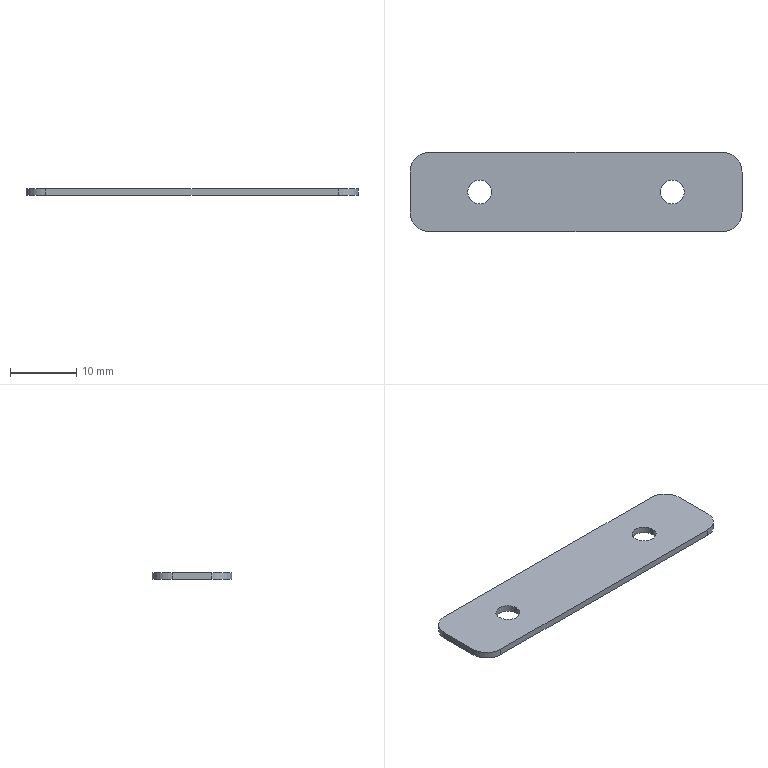Part | NX | features BREP 1 | 1 solid | 14 faces | box 50 x 12 x 1 mm | volume 571.917 mm3 | cylinder 8 | plane 6 | commonest cylinder face diameters 3.6 x4 6 x4
STEP:
#1=CARTESIAN_POINT('',(-22.,6.,1.));
#2=VERTEX_POINT('',#1);
#3=CARTESIAN_POINT('',(-25.,3.,1.));
#4=VERTEX_POINT('',#3);
#5=CARTESIAN_POINT('',(-22.,3.,1.));
#6=DIRECTION('',(0.,0.,1.));
#7=DIRECTION('',(-1.,0.,0.));
#8=AXIS2_PLACEMENT_3D('',#5,#6,#7);
#9=CIRCLE('',#8,3.);
#10=EDGE_CURVE('',#2,#4,#9,.T.);
#11=ORIENTED_EDGE('',*,*,#10,.F.);
#12=CARTESIAN_POINT('',(-22.,6.,0.));
#13=VERTEX_POINT('',#12);
#14=CARTESIAN_POINT('',(-22.,6.,1.));
#15=DIRECTION('',(0.,0.,1.));
#16=VECTOR('',#15,1000.);
#17=LINE('',#14,#16);
#18=EDGE_CURVE('',#13,#2,#17,.T.);
#19=ORIENTED_EDGE('',*,*,#18,.F.);
#20=CARTESIAN_POINT('',(-25.,3.,0.));
#21=VERTEX_POINT('',#20);
#22=CARTESIAN_POINT('',(-22.,3.,0.));
#23=DIRECTION('',(0.,0.,-1.));
#24=DIRECTION('',(-1.,0.,0.));
#25=AXIS2_PLACEMENT_3D('',#22,#23,#24);
#26=CIRCLE('',#25,3.);
#27=EDGE_CURVE('',#21,#13,#26,.T.);
#28=ORIENTED_EDGE('',*,*,#27,.F.);
#29=CARTESIAN_POINT('',(-25.,3.,1.));
#30=DIRECTION('',(0.,0.,-1.));
#31=VECTOR('',#30,1000.);
#32=LINE('',#29,#31);
#33=EDGE_CURVE('',#4,#21,#32,.T.);
#34=ORIENTED_EDGE('',*,*,#33,.F.);
#35=EDGE_LOOP('',(#11,#19,#28,#34));
#36=FACE_BOUND('',#35,.T.);
#37=CARTESIAN_POINT('',(-22.,3.,1.));
#38=DIRECTION('',(0.,0.,-1.));
#39=DIRECTION('',(-1.,0.,0.));
#40=AXIS2_PLACEMENT_3D('',#37,#38,#39);
#41=CYLINDRICAL_SURFACE('',#40,3.);
#42=ADVANCED_FACE('',(#36),#41,.T.);
#43=CARTESIAN_POINT('',(-25.,-3.,1.));
#44=VERTEX_POINT('',#43);
#45=CARTESIAN_POINT('',(-22.,-6.,1.));
#46=VERTEX_POINT('',#45);
#47=CARTESIAN_POINT('',(-22.,-3.,1.));
#48=DIRECTION('',(0.,0.,1.));
#49=DIRECTION('',(-1.,0.,0.));
#50=AXIS2_PLACEMENT_3D('',#47,#48,#49);
#51=CIRCLE('',#50,3.);
#52=EDGE_CURVE('',#44,#46,#51,.T.);
#53=ORIENTED_EDGE('',*,*,#52,.F.);
#54=CARTESIAN_POINT('',(-25.,-3.,0.));
#55=VERTEX_POINT('',#54);
#56=CARTESIAN_POINT('',(-25.,-3.,1.));
#57=DIRECTION('',(0.,0.,1.));
#58=VECTOR('',#57,1000.);
#59=LINE('',#56,#58);
#60=EDGE_CURVE('',#55,#44,#59,.T.);
#61=ORIENTED_EDGE('',*,*,#60,.F.);
#62=CARTESIAN_POINT('',(-22.,-6.,0.));
#63=VERTEX_POINT('',#62);
#64=CARTESIAN_POINT('',(-22.,-3.,0.));
#65=DIRECTION('',(0.,0.,-1.));
#66=DIRECTION('',(-1.,0.,0.));
#67=AXIS2_PLACEMENT_3D('',#64,#65,#66);
#68=CIRCLE('',#67,3.);
#69=EDGE_CURVE('',#63,#55,#68,.T.);
#70=ORIENTED_EDGE('',*,*,#69,.F.);
#71=CARTESIAN_POINT('',(-22.,-6.,1.));
#72=DIRECTION('',(0.,0.,-1.));
#73=VECTOR('',#72,1000.);
#74=LINE('',#71,#73);
#75=EDGE_CURVE('',#46,#63,#74,.T.);
#76=ORIENTED_EDGE('',*,*,#75,.F.);
#77=EDGE_LOOP('',(#53,#61,#70,#76));
#78=FACE_BOUND('',#77,.T.);
#79=CARTESIAN_POINT('',(-22.,-3.,1.));
#80=DIRECTION('',(0.,0.,-1.));
#81=DIRECTION('',(-1.,0.,0.));
#82=AXIS2_PLACEMENT_3D('',#79,#80,#81);
#83=CYLINDRICAL_SURFACE('',#82,3.);
#84=ADVANCED_FACE('',(#78),#83,.T.);
#85=CARTESIAN_POINT('',(25.,3.,1.));
#86=VERTEX_POINT('',#85);
#87=CARTESIAN_POINT('',(22.,6.,1.));
#88=VERTEX_POINT('',#87);
#89=CARTESIAN_POINT('',(22.,3.,1.));
#90=DIRECTION('',(0.,0.,1.));
#91=DIRECTION('',(-1.,0.,0.));
#92=AXIS2_PLACEMENT_3D('',#89,#90,#91);
#93=CIRCLE('',#92,3.);
#94=EDGE_CURVE('',#86,#88,#93,.T.);
#95=ORIENTED_EDGE('',*,*,#94,.F.);
#96=CARTESIAN_POINT('',(25.,3.,0.));
#97=VERTEX_POINT('',#96);
#98=CARTESIAN_POINT('',(25.,3.,1.));
#99=DIRECTION('',(0.,0.,1.));
#100=VECTOR('',#99,1000.);
#101=LINE('',#98,#100);
#102=EDGE_CURVE('',#97,#86,#101,.T.);
#103=ORIENTED_EDGE('',*,*,#102,.F.);
#104=CARTESIAN_POINT('',(22.,6.,0.));
#105=VERTEX_POINT('',#104);
#106=CARTESIAN_POINT('',(22.,3.,0.));
#107=DIRECTION('',(0.,0.,-1.));
#108=DIRECTION('',(-1.,0.,0.));
#109=AXIS2_PLACEMENT_3D('',#106,#107,#108);
#110=CIRCLE('',#109,3.);
#111=EDGE_CURVE('',#105,#97,#110,.T.);
#112=ORIENTED_EDGE('',*,*,#111,.F.);
#113=CARTESIAN_POINT('',(22.,6.,1.));
#114=DIRECTION('',(0.,0.,-1.));
#115=VECTOR('',#114,1000.);
#116=LINE('',#113,#115);
#117=EDGE_CURVE('',#88,#105,#116,.T.);
#118=ORIENTED_EDGE('',*,*,#117,.F.);
#119=EDGE_LOOP('',(#95,#103,#112,#118));
#120=FACE_BOUND('',#119,.T.);
#121=CARTESIAN_POINT('',(22.,3.,1.));
#122=DIRECTION('',(0.,0.,-1.));
#123=DIRECTION('',(-1.,0.,0.));
#124=AXIS2_PLACEMENT_3D('',#121,#122,#123);
#125=CYLINDRICAL_SURFACE('',#124,3.);
#126=ADVANCED_FACE('',(#120),#125,.T.);
#127=CARTESIAN_POINT('',(22.,-6.,1.));
#128=VERTEX_POINT('',#127);
#129=CARTESIAN_POINT('',(25.,-3.,1.));
#130=VERTEX_POINT('',#129);
#131=CARTESIAN_POINT('',(22.,-3.,1.));
#132=DIRECTION('',(0.,0.,1.));
#133=DIRECTION('',(-1.,0.,0.));
#134=AXIS2_PLACEMENT_3D('',#131,#132,#133);
#135=CIRCLE('',#134,3.);
#136=EDGE_CURVE('',#128,#130,#135,.T.);
#137=ORIENTED_EDGE('',*,*,#136,.F.);
#138=CARTESIAN_POINT('',(22.,-6.,0.));
#139=VERTEX_POINT('',#138);
#140=CARTESIAN_POINT('',(22.,-6.,1.));
#141=DIRECTION('',(0.,0.,1.));
#142=VECTOR('',#141,1000.);
#143=LINE('',#140,#142);
#144=EDGE_CURVE('',#139,#128,#143,.T.);
#145=ORIENTED_EDGE('',*,*,#144,.F.);
#146=CARTESIAN_POINT('',(25.,-3.,0.));
#147=VERTEX_POINT('',#146);
#148=CARTESIAN_POINT('',(22.,-3.,0.));
#149=DIRECTION('',(0.,0.,-1.));
#150=DIRECTION('',(-1.,0.,0.));
#151=AXIS2_PLACEMENT_3D('',#148,#149,#150);
#152=CIRCLE('',#151,3.);
#153=EDGE_CURVE('',#147,#139,#152,.T.);
#154=ORIENTED_EDGE('',*,*,#153,.F.);
#155=CARTESIAN_POINT('',(25.,-3.,1.));
#156=DIRECTION('',(0.,0.,-1.));
#157=VECTOR('',#156,1000.);
#158=LINE('',#155,#157);
#159=EDGE_CURVE('',#130,#147,#158,.T.);
#160=ORIENTED_EDGE('',*,*,#159,.F.);
#161=EDGE_LOOP('',(#137,#145,#154,#160));
#162=FACE_BOUND('',#161,.T.);
#163=CARTESIAN_POINT('',(22.,-3.,1.));
#164=DIRECTION('',(0.,0.,-1.));
#165=DIRECTION('',(-1.,0.,0.));
#166=AXIS2_PLACEMENT_3D('',#163,#164,#165);
#167=CYLINDRICAL_SURFACE('',#166,3.);
#168=ADVANCED_FACE('',(#162),#167,.T.);
#169=CARTESIAN_POINT('',(12.7,0.,1.));
#170=VERTEX_POINT('',#169);
#171=CARTESIAN_POINT('',(12.7,0.,0.));
#172=VERTEX_POINT('',#171);
#173=CARTESIAN_POINT('',(12.7,0.,0.));
#174=DIRECTION('',(0.,0.,1.));
#175=VECTOR('',#174,1000.);
#176=LINE('',#173,#175);
#177=EDGE_CURVE('',#170,#172,#176,.F.);
#178=ORIENTED_EDGE('',*,*,#177,.T.);
#179=CARTESIAN_POINT('',(16.3,0.,0.));
#180=VERTEX_POINT('',#179);
#181=CARTESIAN_POINT('',(14.5,0.,0.));
#182=DIRECTION('',(0.,0.,1.));
#183=DIRECTION('',(1.,0.,0.));
#184=AXIS2_PLACEMENT_3D('',#181,#182,#183);
#185=CIRCLE('',#184,1.8);
#186=EDGE_CURVE('',#180,#172,#185,.T.);
#187=ORIENTED_EDGE('',*,*,#186,.F.);
#188=CARTESIAN_POINT('',(16.3,0.,1.));
#189=VERTEX_POINT('',#188);
#190=CARTESIAN_POINT('',(16.3,0.,0.));
#191=DIRECTION('',(0.,0.,1.));
#192=VECTOR('',#191,1000.);
#193=LINE('',#190,#192);
#194=EDGE_CURVE('',#189,#180,#193,.F.);
#195=ORIENTED_EDGE('',*,*,#194,.F.);
#196=CARTESIAN_POINT('',(14.5,0.,1.));
#197=DIRECTION('',(0.,0.,1.));
#198=DIRECTION('',(1.,0.,0.));
#199=AXIS2_PLACEMENT_3D('',#196,#197,#198);
#200=CIRCLE('',#199,1.8);
#201=EDGE_CURVE('',#189,#170,#200,.T.);
#202=ORIENTED_EDGE('',*,*,#201,.T.);
#203=EDGE_LOOP('',(#178,#187,#195,#202));
#204=FACE_BOUND('',#203,.T.);
#205=CARTESIAN_POINT('',(14.5,0.,0.));
#206=DIRECTION('',(0.,0.,1.));
#207=DIRECTION('',(1.,0.,0.));
#208=AXIS2_PLACEMENT_3D('',#205,#206,#207);
#209=CYLINDRICAL_SURFACE('',#208,1.8);
#210=ADVANCED_FACE('',(#204),#209,.F.);
#211=CARTESIAN_POINT('',(-16.3,0.,1.));
#212=VERTEX_POINT('',#211);
#213=CARTESIAN_POINT('',(-16.3,0.,0.));
#214=VERTEX_POINT('',#213);
#215=CARTESIAN_POINT('',(-16.3,0.,0.));
#216=DIRECTION('',(0.,0.,1.));
#217=VECTOR('',#216,1000.);
#218=LINE('',#215,#217);
#219=EDGE_CURVE('',#212,#214,#218,.F.);
#220=ORIENTED_EDGE('',*,*,#219,.T.);
#221=CARTESIAN_POINT('',(-12.7,0.,0.));
#222=VERTEX_POINT('',#221);
#223=CARTESIAN_POINT('',(-14.5,0.,0.));
#224=DIRECTION('',(0.,0.,1.));
#225=DIRECTION('',(1.,0.,0.));
#226=AXIS2_PLACEMENT_3D('',#223,#224,#225);
#227=CIRCLE('',#226,1.8);
#228=EDGE_CURVE('',#222,#214,#227,.T.);
#229=ORIENTED_EDGE('',*,*,#228,.F.);
#230=CARTESIAN_POINT('',(-12.7,0.,1.));
#231=VERTEX_POINT('',#230);
#232=CARTESIAN_POINT('',(-12.7,0.,0.));
#233=DIRECTION('',(0.,0.,1.));
#234=VECTOR('',#233,1000.);
#235=LINE('',#232,#234);
#236=EDGE_CURVE('',#231,#222,#235,.F.);
#237=ORIENTED_EDGE('',*,*,#236,.F.);
#238=CARTESIAN_POINT('',(-14.5,0.,1.));
#239=DIRECTION('',(0.,0.,1.));
#240=DIRECTION('',(1.,0.,0.));
#241=AXIS2_PLACEMENT_3D('',#238,#239,#240);
#242=CIRCLE('',#241,1.8);
#243=EDGE_CURVE('',#231,#212,#242,.T.);
#244=ORIENTED_EDGE('',*,*,#243,.T.);
#245=EDGE_LOOP('',(#220,#229,#237,#244));
#246=FACE_BOUND('',#245,.T.);
#247=CARTESIAN_POINT('',(-14.5,0.,0.));
#248=DIRECTION('',(0.,0.,1.));
#249=DIRECTION('',(1.,0.,0.));
#250=AXIS2_PLACEMENT_3D('',#247,#248,#249);
#251=CYLINDRICAL_SURFACE('',#250,1.8);
#252=ADVANCED_FACE('',(#246),#251,.F.);
#253=CARTESIAN_POINT('',(25.,-6.,0.));
#254=DIRECTION('',(0.,1.,0.));
#255=VECTOR('',#254,1000.);
#256=LINE('',#253,#255);
#257=EDGE_CURVE('',#147,#97,#256,.T.);
#258=ORIENTED_EDGE('',*,*,#257,.F.);
#259=ORIENTED_EDGE('',*,*,#153,.T.);
#260=CARTESIAN_POINT('',(-25.,-6.,0.));
#261=DIRECTION('',(1.,0.,0.));
#262=VECTOR('',#261,1000.);
#263=LINE('',#260,#262);
#264=EDGE_CURVE('',#63,#139,#263,.T.);
#265=ORIENTED_EDGE('',*,*,#264,.F.);
#266=ORIENTED_EDGE('',*,*,#69,.T.);
#267=CARTESIAN_POINT('',(-25.,-6.,0.));
#268=DIRECTION('',(0.,-1.,0.));
#269=VECTOR('',#268,1000.);
#270=LINE('',#267,#269);
#271=EDGE_CURVE('',#21,#55,#270,.T.);
#272=ORIENTED_EDGE('',*,*,#271,.F.);
#273=ORIENTED_EDGE('',*,*,#27,.T.);
#274=CARTESIAN_POINT('',(-25.,6.,0.));
#275=DIRECTION('',(-1.,0.,0.));
#276=VECTOR('',#275,1000.);
#277=LINE('',#274,#276);
#278=EDGE_CURVE('',#105,#13,#277,.T.);
#279=ORIENTED_EDGE('',*,*,#278,.F.);
#280=ORIENTED_EDGE('',*,*,#111,.T.);
#281=EDGE_LOOP('',(#258,#259,#265,#266,#272,#273,#279,#280));
#282=FACE_BOUND('',#281,.T.);
#283=ORIENTED_EDGE('',*,*,#228,.T.);
#284=CARTESIAN_POINT('',(-14.5,0.,0.));
#285=DIRECTION('',(0.,0.,1.));
#286=DIRECTION('',(1.,0.,0.));
#287=AXIS2_PLACEMENT_3D('',#284,#285,#286);
#288=CIRCLE('',#287,1.8);
#289=EDGE_CURVE('',#214,#222,#288,.T.);
#290=ORIENTED_EDGE('',*,*,#289,.T.);
#291=EDGE_LOOP('',(#283,#290));
#292=FACE_BOUND('',#291,.T.);
#293=ORIENTED_EDGE('',*,*,#186,.T.);
#294=CARTESIAN_POINT('',(14.5,0.,0.));
#295=DIRECTION('',(0.,0.,1.));
#296=DIRECTION('',(1.,0.,0.));
#297=AXIS2_PLACEMENT_3D('',#294,#295,#296);
#298=CIRCLE('',#297,1.8);
#299=EDGE_CURVE('',#172,#180,#298,.T.);
#300=ORIENTED_EDGE('',*,*,#299,.T.);
#301=EDGE_LOOP('',(#293,#300));
#302=FACE_BOUND('',#301,.T.);
#303=CARTESIAN_POINT('',(25.,6.,0.));
#304=DIRECTION('',(0.,0.,-1.));
#305=DIRECTION('',(-1.,0.,0.));
#306=AXIS2_PLACEMENT_3D('',#303,#304,#305);
#307=PLANE('',#306);
#308=ADVANCED_FACE('',(#282,#292,#302),#307,.T.);
#309=CARTESIAN_POINT('',(-25.,-6.,1.));
#310=DIRECTION('',(1.,0.,0.));
#311=VECTOR('',#310,1000.);
#312=LINE('',#309,#311);
#313=EDGE_CURVE('',#46,#128,#312,.T.);
#314=ORIENTED_EDGE('',*,*,#313,.T.);
#315=ORIENTED_EDGE('',*,*,#136,.T.);
#316=CARTESIAN_POINT('',(25.,-6.,1.));
#317=DIRECTION('',(0.,1.,0.));
#318=VECTOR('',#317,1000.);
#319=LINE('',#316,#318);
#320=EDGE_CURVE('',#130,#86,#319,.T.);
#321=ORIENTED_EDGE('',*,*,#320,.T.);
#322=ORIENTED_EDGE('',*,*,#94,.T.);
#323=CARTESIAN_POINT('',(-25.,6.,1.));
#324=DIRECTION('',(-1.,0.,0.));
#325=VECTOR('',#324,1000.);
#326=LINE('',#323,#325);
#327=EDGE_CURVE('',#88,#2,#326,.T.);
#328=ORIENTED_EDGE('',*,*,#327,.T.);
#329=ORIENTED_EDGE('',*,*,#10,.T.);
#330=CARTESIAN_POINT('',(-25.,-6.,1.));
#331=DIRECTION('',(0.,-1.,0.));
#332=VECTOR('',#331,1000.);
#333=LINE('',#330,#332);
#334=EDGE_CURVE('',#4,#44,#333,.T.);
#335=ORIENTED_EDGE('',*,*,#334,.T.);
#336=ORIENTED_EDGE('',*,*,#52,.T.);
#337=EDGE_LOOP('',(#314,#315,#321,#322,#328,#329,#335,#336));
#338=FACE_BOUND('',#337,.T.);
#339=ORIENTED_EDGE('',*,*,#243,.F.);
#340=CARTESIAN_POINT('',(-14.5,0.,1.));
#341=DIRECTION('',(0.,0.,1.));
#342=DIRECTION('',(1.,0.,0.));
#343=AXIS2_PLACEMENT_3D('',#340,#341,#342);
#344=CIRCLE('',#343,1.8);
#345=EDGE_CURVE('',#212,#231,#344,.T.);
#346=ORIENTED_EDGE('',*,*,#345,.F.);
#347=EDGE_LOOP('',(#339,#346));
#348=FACE_BOUND('',#347,.T.);
#349=ORIENTED_EDGE('',*,*,#201,.F.);
#350=CARTESIAN_POINT('',(14.5,0.,1.));
#351=DIRECTION('',(0.,0.,1.));
#352=DIRECTION('',(1.,0.,0.));
#353=AXIS2_PLACEMENT_3D('',#350,#351,#352);
#354=CIRCLE('',#353,1.8);
#355=EDGE_CURVE('',#170,#189,#354,.T.);
#356=ORIENTED_EDGE('',*,*,#355,.F.);
#357=EDGE_LOOP('',(#349,#356));
#358=FACE_BOUND('',#357,.T.);
#359=CARTESIAN_POINT('',(25.,6.,1.));
#360=DIRECTION('',(0.,0.,-1.));
#361=DIRECTION('',(-1.,0.,0.));
#362=AXIS2_PLACEMENT_3D('',#359,#360,#361);
#363=PLANE('',#362);
#364=ADVANCED_FACE('',(#338,#348,#358),#363,.F.);
#365=ORIENTED_EDGE('',*,*,#264,.T.);
#366=ORIENTED_EDGE('',*,*,#144,.T.);
#367=ORIENTED_EDGE('',*,*,#313,.F.);
#368=ORIENTED_EDGE('',*,*,#75,.T.);
#369=EDGE_LOOP('',(#365,#366,#367,#368));
#370=FACE_BOUND('',#369,.T.);
#371=CARTESIAN_POINT('',(-25.,-6.,1.));
#372=DIRECTION('',(0.,1.,0.));
#373=DIRECTION('',(0.,0.,1.));
#374=AXIS2_PLACEMENT_3D('',#371,#372,#373);
#375=PLANE('',#374);
#376=ADVANCED_FACE('',(#370),#375,.F.);
#377=ORIENTED_EDGE('',*,*,#271,.T.);
#378=ORIENTED_EDGE('',*,*,#60,.T.);
#379=ORIENTED_EDGE('',*,*,#334,.F.);
#380=ORIENTED_EDGE('',*,*,#33,.T.);
#381=EDGE_LOOP('',(#377,#378,#379,#380));
#382=FACE_BOUND('',#381,.T.);
#383=CARTESIAN_POINT('',(-25.,-6.,1.));
#384=DIRECTION('',(1.,0.,0.));
#385=DIRECTION('',(0.,0.,-1.));
#386=AXIS2_PLACEMENT_3D('',#383,#384,#385);
#387=PLANE('',#386);
#388=ADVANCED_FACE('',(#382),#387,.F.);
#389=ORIENTED_EDGE('',*,*,#327,.F.);
#390=ORIENTED_EDGE('',*,*,#117,.T.);
#391=ORIENTED_EDGE('',*,*,#278,.T.);
#392=ORIENTED_EDGE('',*,*,#18,.T.);
#393=EDGE_LOOP('',(#389,#390,#391,#392));
#394=FACE_BOUND('',#393,.T.);
#395=CARTESIAN_POINT('',(-25.,6.,1.));
#396=DIRECTION('',(0.,-1.,0.));
#397=DIRECTION('',(0.,0.,-1.));
#398=AXIS2_PLACEMENT_3D('',#395,#396,#397);
#399=PLANE('',#398);
#400=ADVANCED_FACE('',(#394),#399,.F.);
#401=ORIENTED_EDGE('',*,*,#320,.F.);
#402=ORIENTED_EDGE('',*,*,#159,.T.);
#403=ORIENTED_EDGE('',*,*,#257,.T.);
#404=ORIENTED_EDGE('',*,*,#102,.T.);
#405=EDGE_LOOP('',(#401,#402,#403,#404));
#406=FACE_BOUND('',#405,.T.);
#407=CARTESIAN_POINT('',(25.,-6.,1.));
#408=DIRECTION('',(-1.,0.,0.));
#409=DIRECTION('',(0.,0.,1.));
#410=AXIS2_PLACEMENT_3D('',#407,#408,#409);
#411=PLANE('',#410);
#412=ADVANCED_FACE('',(#406),#411,.F.);
#413=ORIENTED_EDGE('',*,*,#289,.F.);
#414=ORIENTED_EDGE('',*,*,#219,.F.);
#415=ORIENTED_EDGE('',*,*,#345,.T.);
#416=ORIENTED_EDGE('',*,*,#236,.T.);
#417=EDGE_LOOP('',(#413,#414,#415,#416));
#418=FACE_BOUND('',#417,.T.);
#419=CARTESIAN_POINT('',(-14.5,0.,0.));
#420=DIRECTION('',(0.,0.,1.));
#421=DIRECTION('',(1.,0.,0.));
#422=AXIS2_PLACEMENT_3D('',#419,#420,#421);
#423=CYLINDRICAL_SURFACE('',#422,1.8);
#424=ADVANCED_FACE('',(#418),#423,.F.);
#425=ORIENTED_EDGE('',*,*,#299,.F.);
#426=ORIENTED_EDGE('',*,*,#177,.F.);
#427=ORIENTED_EDGE('',*,*,#355,.T.);
#428=ORIENTED_EDGE('',*,*,#194,.T.);
#429=EDGE_LOOP('',(#425,#426,#427,#428));
#430=FACE_BOUND('',#429,.T.);
#431=CARTESIAN_POINT('',(14.5,0.,0.));
#432=DIRECTION('',(0.,0.,1.));
#433=DIRECTION('',(1.,0.,0.));
#434=AXIS2_PLACEMENT_3D('',#431,#432,#433);
#435=CYLINDRICAL_SURFACE('',#434,1.8);
#436=ADVANCED_FACE('',(#430),#435,.F.);
#437=CLOSED_SHELL('',(#42,#84,#126,#168,#210,#252,#308,#364,#376,#388,#400,#412,#424,#436));
#438=MANIFOLD_SOLID_BREP('',#437);
#439=(LENGTH_UNIT()NAMED_UNIT(*)SI_UNIT(.MILLI.,.METRE.));
#440=UNCERTAINTY_MEASURE_WITH_UNIT(LENGTH_MEASURE(0.00001),#439,'','');
#441=(NAMED_UNIT(*)PLANE_ANGLE_UNIT()SI_UNIT($,.RADIAN.));
#442=(NAMED_UNIT(*)SI_UNIT($,.STERADIAN.)SOLID_ANGLE_UNIT());
#443=(GEOMETRIC_REPRESENTATION_CONTEXT(3)GLOBAL_UNCERTAINTY_ASSIGNED_CONTEXT((#440))GLOBAL_UNIT_ASSIGNED_CONTEXT((#439,#441,#442))REPRESENTATION_CONTEXT('',''));
#444=ADVANCED_BREP_SHAPE_REPRESENTATION('',(#438),#443);